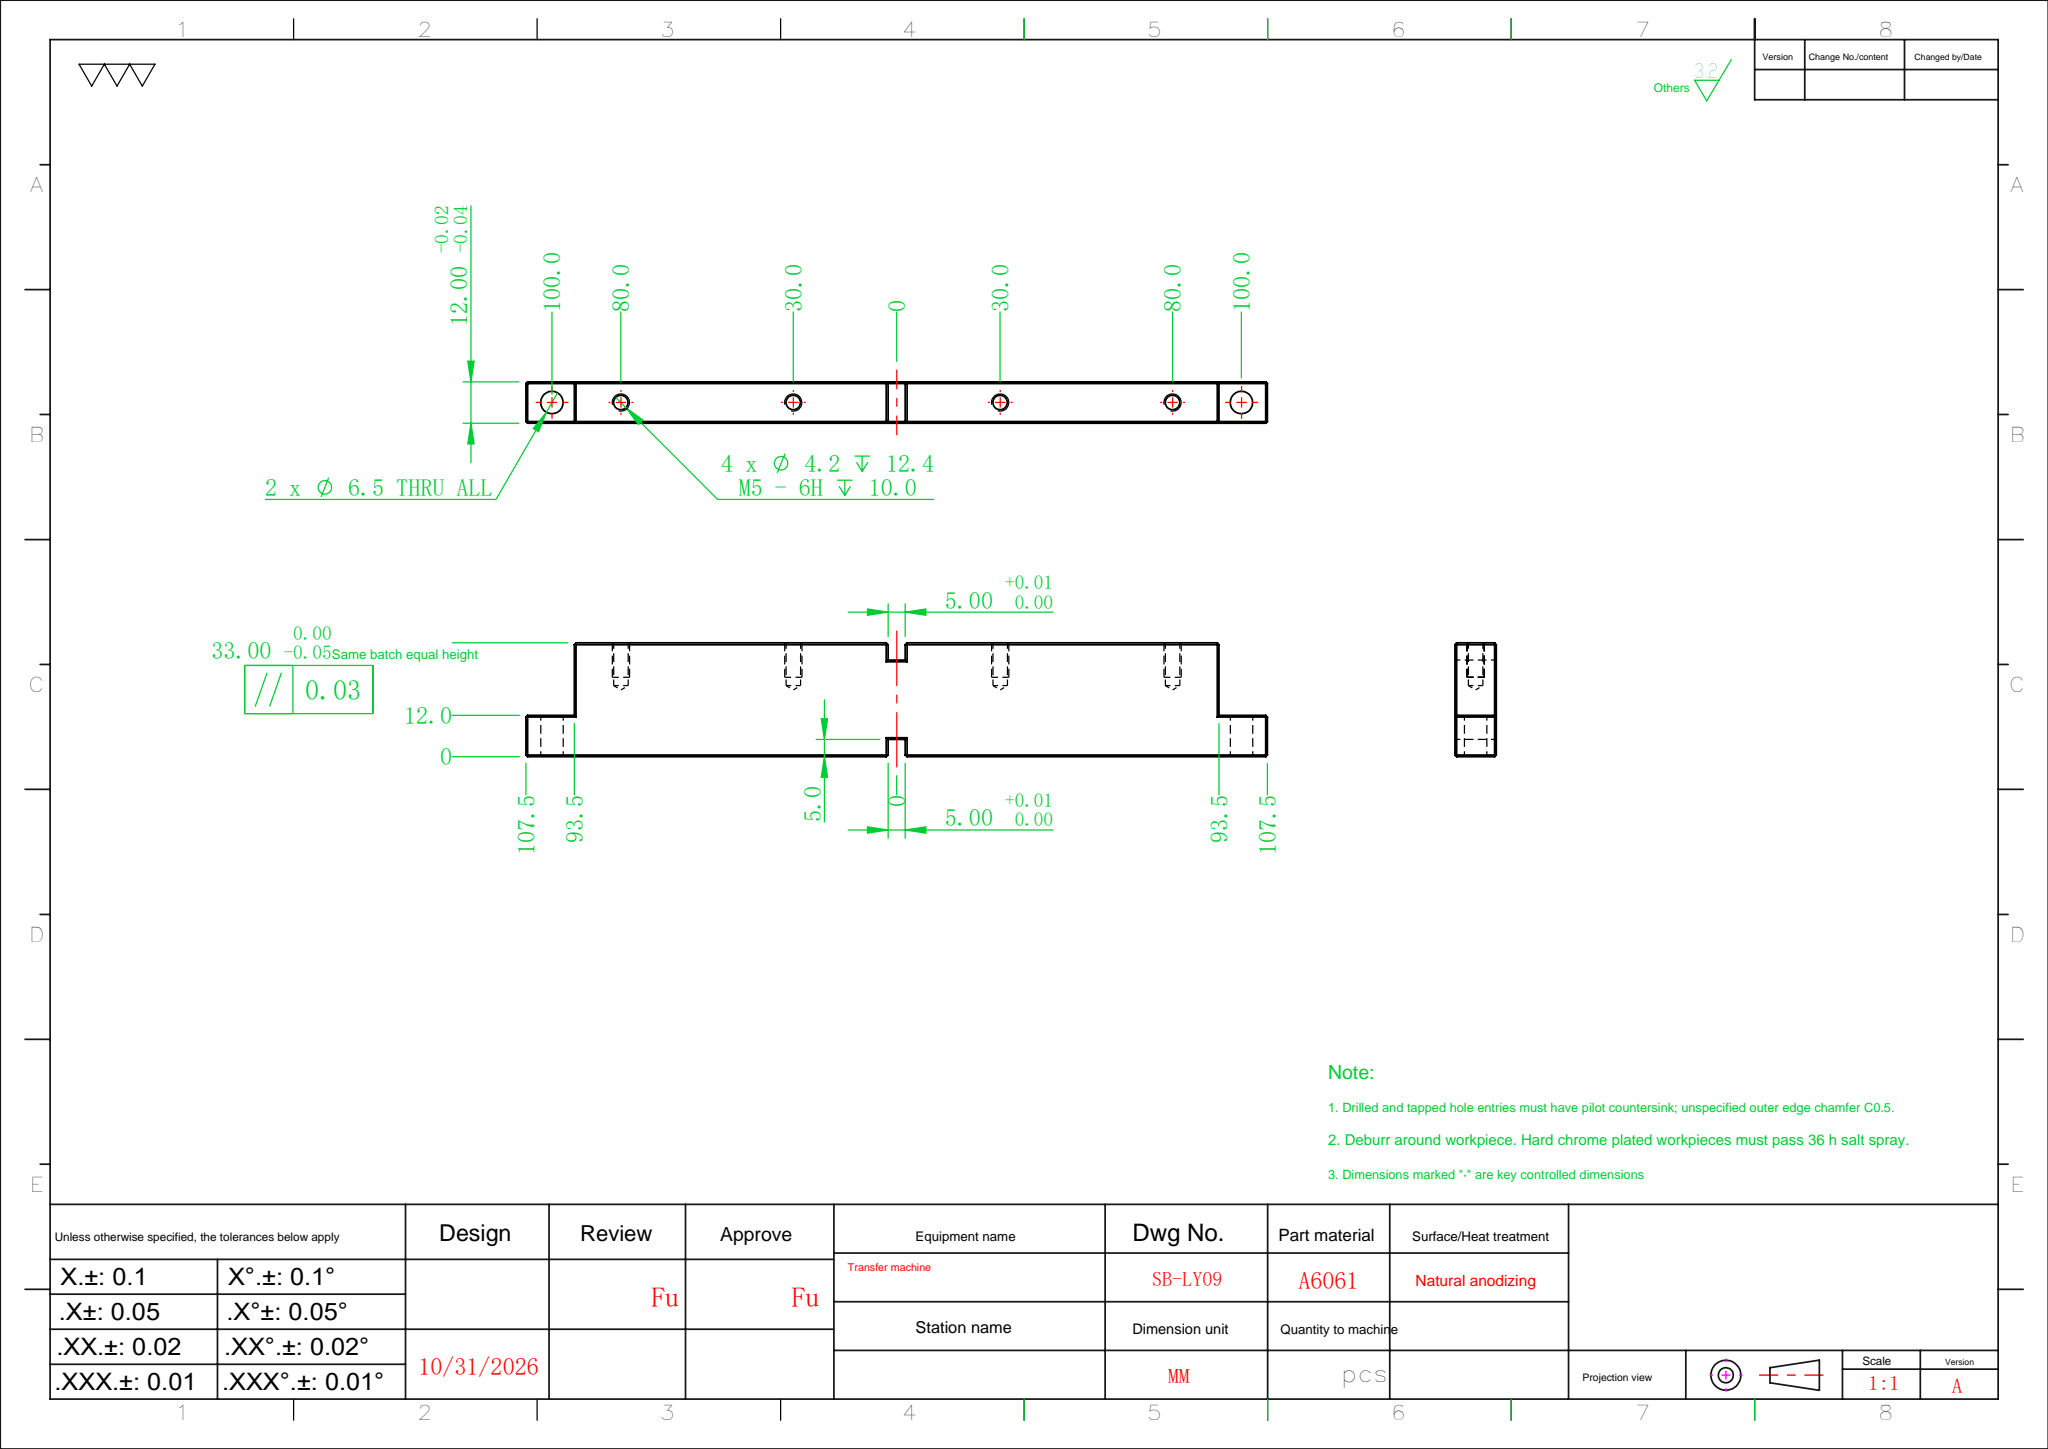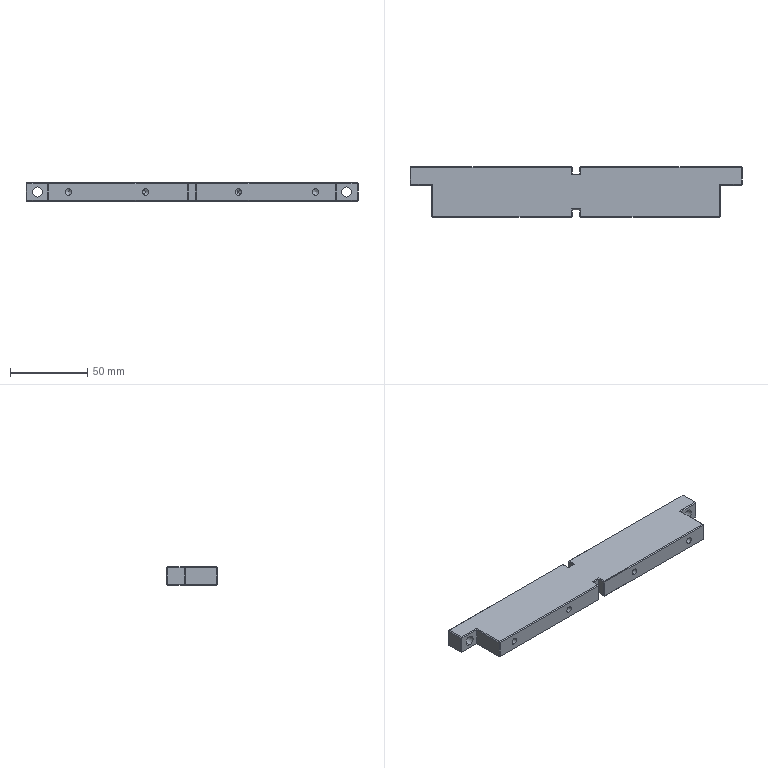Part | SolidWorks | features ICE 3, HoleWzd 2, Chamfer 1, Extrusion 1 | 1 solid | 100 faces | box 215 x 33 x 12 mm | volume 75834 mm3 | plane 80 | cylinder 12 | cone 8 | commonest cylinder face diameters 4.2 x8 6.5 x4